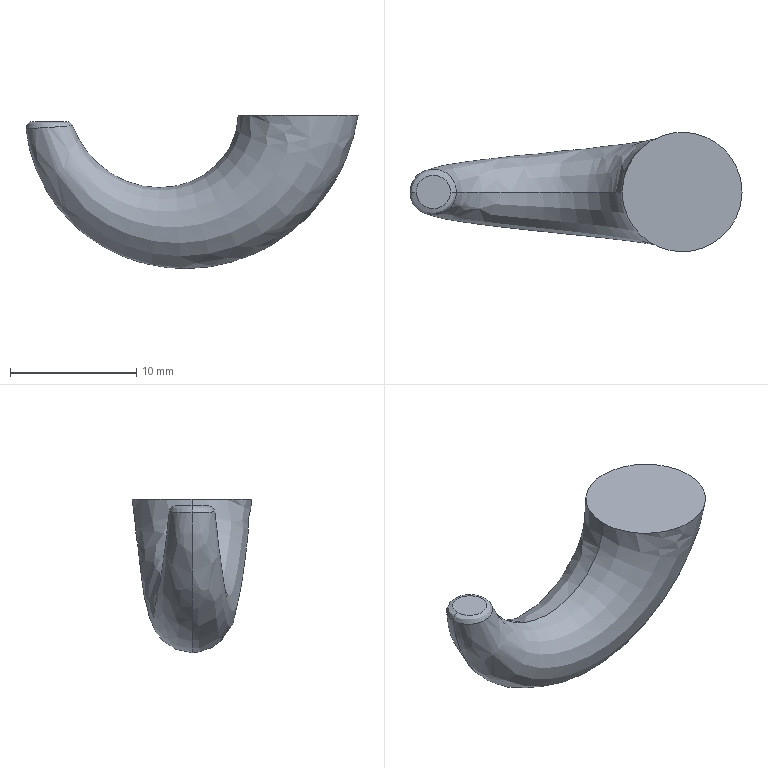Part | STEP file | solid 219 | 1 solid | 6 faces | volume 1019 mm3 | spline 4 | plane 2